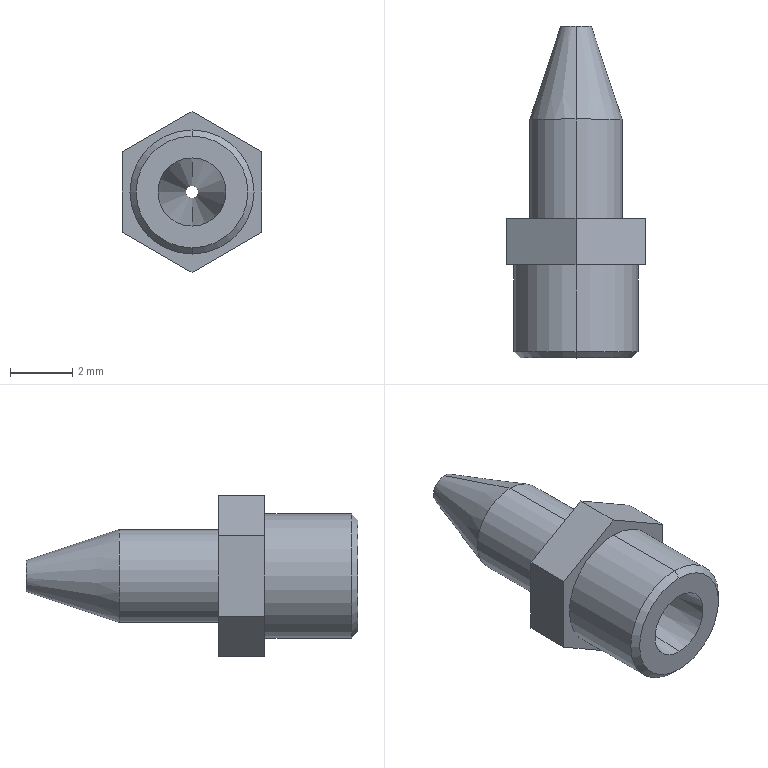Part | SolidWorks | features ICE 4, Chamfer 2, Extrusion 1, RevCut 1 | 1 solid | 20 faces | box 4.5 x 10.7 x 5.196 mm | volume 80.12 mm3 | plane 10 | cone 6 | cylinder 4 | commonest cylinder face diameters 3 x2 4 x2
STEP:
#1=CARTESIAN_POINT('',(0.,-4.5,-1.8));
#2=VERTEX_POINT('',#1);
#3=CARTESIAN_POINT('',(0.,-4.5,1.8));
#4=VERTEX_POINT('',#3);
#5=CARTESIAN_POINT('',(0.,-4.5,0.));
#6=DIRECTION('',(0.,-1.,0.));
#7=DIRECTION('',(0.,0.,-1.));
#8=AXIS2_PLACEMENT_3D('',#5,#6,#7);
#9=CIRCLE('',#8,1.8);
#10=EDGE_CURVE('',#2,#4,#9,.T.);
#11=ORIENTED_EDGE('',*,*,#10,.F.);
#12=CARTESIAN_POINT('',(0.,-4.3,-2.));
#13=VERTEX_POINT('',#12);
#14=CARTESIAN_POINT('',(0.,-4.5,-1.8));
#15=DIRECTION('',(0.,0.7071,-0.7071));
#16=VECTOR('',#15,1000.);
#17=LINE('',#14,#16);
#18=EDGE_CURVE('',#2,#13,#17,.T.);
#19=ORIENTED_EDGE('',*,*,#18,.T.);
#20=CARTESIAN_POINT('',(0.,-4.3,2.));
#21=VERTEX_POINT('',#20);
#22=CARTESIAN_POINT('',(0.,-4.3,0.));
#23=DIRECTION('',(0.,1.,0.));
#24=DIRECTION('',(0.,0.,-1.));
#25=AXIS2_PLACEMENT_3D('',#22,#23,#24);
#26=CIRCLE('',#25,2.);
#27=EDGE_CURVE('',#21,#13,#26,.T.);
#28=ORIENTED_EDGE('',*,*,#27,.F.);
#29=CARTESIAN_POINT('',(0.,-4.5,1.8));
#30=DIRECTION('',(0.,0.7071,0.7071));
#31=VECTOR('',#30,1000.);
#32=LINE('',#29,#31);
#33=EDGE_CURVE('',#4,#21,#32,.T.);
#34=ORIENTED_EDGE('',*,*,#33,.F.);
#35=EDGE_LOOP('',(#11,#19,#28,#34));
#36=FACE_OUTER_BOUND('',#35,.T.);
#37=CARTESIAN_POINT('',(0.,-4.5,0.));
#38=DIRECTION('',(0.,1.,0.));
#39=DIRECTION('',(0.,0.,1.));
#40=AXIS2_PLACEMENT_3D('',#37,#38,#39);
#41=CONICAL_SURFACE('',#40,1.8,0.7854);
#42=ADVANCED_FACE('',(#36),#41,.T.);
#43=CARTESIAN_POINT('',(0.,6.2,0.2));
#44=VERTEX_POINT('',#43);
#45=CARTESIAN_POINT('',(0.,6.2,-0.2));
#46=VERTEX_POINT('',#45);
#47=CARTESIAN_POINT('',(0.,6.2,0.));
#48=DIRECTION('',(0.,-1.,0.));
#49=DIRECTION('',(0.,0.,-1.));
#50=AXIS2_PLACEMENT_3D('',#47,#48,#49);
#51=CIRCLE('',#50,0.2);
#52=EDGE_CURVE('',#44,#46,#51,.T.);
#53=ORIENTED_EDGE('',*,*,#52,.F.);
#54=CARTESIAN_POINT('',(0.,-4.5,1.1));
#55=VERTEX_POINT('',#54);
#56=CARTESIAN_POINT('',(0.,-4.5,1.1));
#57=DIRECTION('',(0.,-0.9965,0.08382));
#58=VECTOR('',#57,1000.);
#59=LINE('',#56,#58);
#60=EDGE_CURVE('',#44,#55,#59,.T.);
#61=ORIENTED_EDGE('',*,*,#60,.T.);
#62=CARTESIAN_POINT('',(0.,-4.5,-1.1));
#63=VERTEX_POINT('',#62);
#64=CARTESIAN_POINT('',(0.,-4.5,0.));
#65=DIRECTION('',(0.,-1.,0.));
#66=DIRECTION('',(0.,0.,-1.));
#67=AXIS2_PLACEMENT_3D('',#64,#65,#66);
#68=CIRCLE('',#67,1.1);
#69=EDGE_CURVE('',#55,#63,#68,.T.);
#70=ORIENTED_EDGE('',*,*,#69,.T.);
#71=CARTESIAN_POINT('',(0.,-4.5,-1.1));
#72=DIRECTION('',(0.,-0.9965,-0.08382));
#73=VECTOR('',#72,1000.);
#74=LINE('',#71,#73);
#75=EDGE_CURVE('',#46,#63,#74,.T.);
#76=ORIENTED_EDGE('',*,*,#75,.F.);
#77=EDGE_LOOP('',(#53,#61,#70,#76));
#78=FACE_OUTER_BOUND('',#77,.T.);
#79=CARTESIAN_POINT('',(0.,-4.5,0.));
#80=DIRECTION('',(0.,-1.,0.));
#81=DIRECTION('',(0.,0.,-1.));
#82=AXIS2_PLACEMENT_3D('',#79,#80,#81);
#83=CONICAL_SURFACE('',#82,1.1,0.08391);
#84=ADVANCED_FACE('',(#78),#83,.F.);
#85=ORIENTED_EDGE('',*,*,#27,.T.);
#86=CARTESIAN_POINT('',(0.,-1.5,-2.));
#87=VERTEX_POINT('',#86);
#88=CARTESIAN_POINT('',(0.,-4.5,-2.));
#89=DIRECTION('',(0.,1.,0.));
#90=VECTOR('',#89,1000.);
#91=LINE('',#88,#90);
#92=EDGE_CURVE('',#13,#87,#91,.T.);
#93=ORIENTED_EDGE('',*,*,#92,.T.);
#94=CARTESIAN_POINT('',(0.,-1.5,2.));
#95=VERTEX_POINT('',#94);
#96=CARTESIAN_POINT('',(0.,-1.5,0.));
#97=DIRECTION('',(0.,-1.,0.));
#98=DIRECTION('',(0.,0.,-1.));
#99=AXIS2_PLACEMENT_3D('',#96,#97,#98);
#100=CIRCLE('',#99,2.);
#101=EDGE_CURVE('',#87,#95,#100,.T.);
#102=ORIENTED_EDGE('',*,*,#101,.T.);
#103=CARTESIAN_POINT('',(0.,-4.5,2.));
#104=DIRECTION('',(0.,1.,0.));
#105=VECTOR('',#104,1000.);
#106=LINE('',#103,#105);
#107=EDGE_CURVE('',#21,#95,#106,.T.);
#108=ORIENTED_EDGE('',*,*,#107,.F.);
#109=EDGE_LOOP('',(#85,#93,#102,#108));
#110=FACE_OUTER_BOUND('',#109,.T.);
#111=CARTESIAN_POINT('',(0.,-4.5,0.));
#112=DIRECTION('',(0.,1.,0.));
#113=DIRECTION('',(0.,0.,1.));
#114=AXIS2_PLACEMENT_3D('',#111,#112,#113);
#115=CYLINDRICAL_SURFACE('',#114,2.);
#116=ADVANCED_FACE('',(#110),#115,.T.);
#117=CARTESIAN_POINT('',(0.,6.2,0.5));
#118=VERTEX_POINT('',#117);
#119=CARTESIAN_POINT('',(0.,6.2,-0.5));
#120=VERTEX_POINT('',#119);
#121=CARTESIAN_POINT('',(0.,6.2,0.));
#122=DIRECTION('',(0.,1.,0.));
#123=DIRECTION('',(0.,0.,1.));
#124=AXIS2_PLACEMENT_3D('',#121,#122,#123);
#125=CIRCLE('',#124,0.5);
#126=EDGE_CURVE('',#118,#120,#125,.T.);
#127=ORIENTED_EDGE('',*,*,#126,.F.);
#128=CARTESIAN_POINT('',(0.,3.2,1.5));
#129=VERTEX_POINT('',#128);
#130=CARTESIAN_POINT('',(0.,6.2,0.5));
#131=DIRECTION('',(0.,-0.9487,0.3162));
#132=VECTOR('',#131,1000.);
#133=LINE('',#130,#132);
#134=EDGE_CURVE('',#118,#129,#133,.T.);
#135=ORIENTED_EDGE('',*,*,#134,.T.);
#136=CARTESIAN_POINT('',(0.,3.2,-1.5));
#137=VERTEX_POINT('',#136);
#138=CARTESIAN_POINT('',(0.,3.2,0.));
#139=DIRECTION('',(0.,-1.,0.));
#140=DIRECTION('',(0.,0.,1.));
#141=AXIS2_PLACEMENT_3D('',#138,#139,#140);
#142=CIRCLE('',#141,1.5);
#143=EDGE_CURVE('',#137,#129,#142,.T.);
#144=ORIENTED_EDGE('',*,*,#143,.F.);
#145=CARTESIAN_POINT('',(0.,6.2,-0.5));
#146=DIRECTION('',(0.,-0.9487,-0.3162));
#147=VECTOR('',#146,1000.);
#148=LINE('',#145,#147);
#149=EDGE_CURVE('',#120,#137,#148,.T.);
#150=ORIENTED_EDGE('',*,*,#149,.F.);
#151=EDGE_LOOP('',(#127,#135,#144,#150));
#152=FACE_OUTER_BOUND('',#151,.T.);
#153=CARTESIAN_POINT('',(0.,6.2,0.));
#154=DIRECTION('',(0.,-1.,0.));
#155=DIRECTION('',(0.,0.,-1.));
#156=AXIS2_PLACEMENT_3D('',#153,#154,#155);
#157=CONICAL_SURFACE('',#156,0.5,0.3218);
#158=ADVANCED_FACE('',(#152),#157,.T.);
#159=ORIENTED_EDGE('',*,*,#143,.T.);
#160=CARTESIAN_POINT('',(0.,0.,1.5));
#161=VERTEX_POINT('',#160);
#162=CARTESIAN_POINT('',(0.,6.2,1.5));
#163=DIRECTION('',(0.,-1.,0.));
#164=VECTOR('',#163,1000.);
#165=LINE('',#162,#164);
#166=EDGE_CURVE('',#129,#161,#165,.T.);
#167=ORIENTED_EDGE('',*,*,#166,.T.);
#168=CARTESIAN_POINT('',(0.,0.,-1.5));
#169=VERTEX_POINT('',#168);
#170=CARTESIAN_POINT('',(0.,0.,0.));
#171=DIRECTION('',(0.,-1.,0.));
#172=DIRECTION('',(0.,0.,-1.));
#173=AXIS2_PLACEMENT_3D('',#170,#171,#172);
#174=CIRCLE('',#173,1.5);
#175=EDGE_CURVE('',#169,#161,#174,.T.);
#176=ORIENTED_EDGE('',*,*,#175,.F.);
#177=CARTESIAN_POINT('',(0.,6.2,-1.5));
#178=DIRECTION('',(0.,-1.,0.));
#179=VECTOR('',#178,1000.);
#180=LINE('',#177,#179);
#181=EDGE_CURVE('',#137,#169,#180,.T.);
#182=ORIENTED_EDGE('',*,*,#181,.F.);
#183=EDGE_LOOP('',(#159,#167,#176,#182));
#184=FACE_OUTER_BOUND('',#183,.T.);
#185=CARTESIAN_POINT('',(0.,6.2,0.));
#186=DIRECTION('',(0.,-1.,0.));
#187=DIRECTION('',(0.,0.,-1.));
#188=AXIS2_PLACEMENT_3D('',#185,#186,#187);
#189=CYLINDRICAL_SURFACE('',#188,1.5);
#190=ADVANCED_FACE('',(#184),#189,.T.);
#191=CARTESIAN_POINT('',(2.25,-1.5,1.299));
#192=VERTEX_POINT('',#191);
#193=CARTESIAN_POINT('',(0.,-1.5,2.598));
#194=VERTEX_POINT('',#193);
#195=CARTESIAN_POINT('',(2.25,-1.5,1.299));
#196=DIRECTION('',(-0.866,0.,0.5));
#197=VECTOR('',#196,1000.);
#198=LINE('',#195,#197);
#199=EDGE_CURVE('',#192,#194,#198,.T.);
#200=ORIENTED_EDGE('',*,*,#199,.T.);
#201=CARTESIAN_POINT('',(-2.25,-1.5,1.299));
#202=VERTEX_POINT('',#201);
#203=CARTESIAN_POINT('',(0.,-1.5,2.598));
#204=DIRECTION('',(-0.866,0.,-0.5));
#205=VECTOR('',#204,1000.);
#206=LINE('',#203,#205);
#207=EDGE_CURVE('',#194,#202,#206,.T.);
#208=ORIENTED_EDGE('',*,*,#207,.T.);
#209=CARTESIAN_POINT('',(-2.25,-1.5,-1.299));
#210=VERTEX_POINT('',#209);
#211=CARTESIAN_POINT('',(-2.25,-1.5,1.299));
#212=DIRECTION('',(0.,0.,-1.));
#213=VECTOR('',#212,1000.);
#214=LINE('',#211,#213);
#215=EDGE_CURVE('',#202,#210,#214,.T.);
#216=ORIENTED_EDGE('',*,*,#215,.T.);
#217=CARTESIAN_POINT('',(0.,-1.5,-2.598));
#218=VERTEX_POINT('',#217);
#219=CARTESIAN_POINT('',(-2.25,-1.5,-1.299));
#220=DIRECTION('',(0.866,0.,-0.5));
#221=VECTOR('',#220,1000.);
#222=LINE('',#219,#221);
#223=EDGE_CURVE('',#210,#218,#222,.T.);
#224=ORIENTED_EDGE('',*,*,#223,.T.);
#225=CARTESIAN_POINT('',(2.25,-1.5,-1.299));
#226=VERTEX_POINT('',#225);
#227=CARTESIAN_POINT('',(0.,-1.5,-2.598));
#228=DIRECTION('',(0.866,0.,0.5));
#229=VECTOR('',#228,1000.);
#230=LINE('',#227,#229);
#231=EDGE_CURVE('',#218,#226,#230,.T.);
#232=ORIENTED_EDGE('',*,*,#231,.T.);
#233=CARTESIAN_POINT('',(2.25,-1.5,-1.299));
#234=DIRECTION('',(0.,0.,1.));
#235=VECTOR('',#234,1000.);
#236=LINE('',#233,#235);
#237=EDGE_CURVE('',#226,#192,#236,.T.);
#238=ORIENTED_EDGE('',*,*,#237,.T.);
#239=EDGE_LOOP('',(#200,#208,#216,#224,#232,#238));
#240=FACE_OUTER_BOUND('',#239,.T.);
#241=CARTESIAN_POINT('',(0.,-1.5,0.));
#242=DIRECTION('',(0.,-1.,0.));
#243=DIRECTION('',(0.,0.,-1.));
#244=AXIS2_PLACEMENT_3D('',#241,#242,#243);
#245=CIRCLE('',#244,2.);
#246=EDGE_CURVE('',#95,#87,#245,.T.);
#247=ORIENTED_EDGE('',*,*,#246,.F.);
#248=ORIENTED_EDGE('',*,*,#101,.F.);
#249=EDGE_LOOP('',(#247,#248));
#250=FACE_BOUND('',#249,.T.);
#251=CARTESIAN_POINT('',(0.,-1.5,0.));
#252=DIRECTION('',(0.,-1.,0.));
#253=DIRECTION('',(0.,0.,-1.));
#254=AXIS2_PLACEMENT_3D('',#251,#252,#253);
#255=PLANE('',#254);
#256=ADVANCED_FACE('',(#240,#250),#255,.T.);
#257=ORIENTED_EDGE('',*,*,#166,.F.);
#258=CARTESIAN_POINT('',(0.,3.2,0.));
#259=DIRECTION('',(0.,-1.,0.));
#260=DIRECTION('',(0.,0.,1.));
#261=AXIS2_PLACEMENT_3D('',#258,#259,#260);
#262=CIRCLE('',#261,1.5);
#263=EDGE_CURVE('',#129,#137,#262,.T.);
#264=ORIENTED_EDGE('',*,*,#263,.T.);
#265=ORIENTED_EDGE('',*,*,#181,.T.);
#266=CARTESIAN_POINT('',(0.,0.,0.));
#267=DIRECTION('',(0.,-1.,0.));
#268=DIRECTION('',(0.,0.,-1.));
#269=AXIS2_PLACEMENT_3D('',#266,#267,#268);
#270=CIRCLE('',#269,1.5);
#271=EDGE_CURVE('',#161,#169,#270,.T.);
#272=ORIENTED_EDGE('',*,*,#271,.F.);
#273=EDGE_LOOP('',(#257,#264,#265,#272));
#274=FACE_OUTER_BOUND('',#273,.T.);
#275=CARTESIAN_POINT('',(0.,6.2,0.));
#276=DIRECTION('',(0.,-1.,0.));
#277=DIRECTION('',(0.,0.,-1.));
#278=AXIS2_PLACEMENT_3D('',#275,#276,#277);
#279=CYLINDRICAL_SURFACE('',#278,1.5);
#280=ADVANCED_FACE('',(#274),#279,.T.);
#281=CARTESIAN_POINT('',(0.,6.2,0.));
#282=DIRECTION('',(0.,1.,0.));
#283=DIRECTION('',(0.,0.,1.));
#284=AXIS2_PLACEMENT_3D('',#281,#282,#283);
#285=CIRCLE('',#284,0.5);
#286=EDGE_CURVE('',#120,#118,#285,.T.);
#287=ORIENTED_EDGE('',*,*,#286,.T.);
#288=ORIENTED_EDGE('',*,*,#126,.T.);
#289=EDGE_LOOP('',(#287,#288));
#290=FACE_OUTER_BOUND('',#289,.T.);
#291=CARTESIAN_POINT('',(0.,6.2,0.));
#292=DIRECTION('',(0.,-1.,0.));
#293=DIRECTION('',(0.,0.,-1.));
#294=AXIS2_PLACEMENT_3D('',#291,#292,#293);
#295=CIRCLE('',#294,0.2);
#296=EDGE_CURVE('',#46,#44,#295,.T.);
#297=ORIENTED_EDGE('',*,*,#296,.T.);
#298=ORIENTED_EDGE('',*,*,#52,.T.);
#299=EDGE_LOOP('',(#297,#298));
#300=FACE_BOUND('',#299,.T.);
#301=CARTESIAN_POINT('',(0.,6.2,0.));
#302=DIRECTION('',(0.,1.,0.));
#303=DIRECTION('',(0.,0.,1.));
#304=AXIS2_PLACEMENT_3D('',#301,#302,#303);
#305=PLANE('',#304);
#306=ADVANCED_FACE('',(#290,#300),#305,.T.);
#307=ORIENTED_EDGE('',*,*,#134,.F.);
#308=ORIENTED_EDGE('',*,*,#286,.F.);
#309=ORIENTED_EDGE('',*,*,#149,.T.);
#310=ORIENTED_EDGE('',*,*,#263,.F.);
#311=EDGE_LOOP('',(#307,#308,#309,#310));
#312=FACE_OUTER_BOUND('',#311,.T.);
#313=CARTESIAN_POINT('',(0.,6.2,0.));
#314=DIRECTION('',(0.,-1.,0.));
#315=DIRECTION('',(0.,0.,-1.));
#316=AXIS2_PLACEMENT_3D('',#313,#314,#315);
#317=CONICAL_SURFACE('',#316,0.5,0.3218);
#318=ADVANCED_FACE('',(#312),#317,.T.);
#319=CARTESIAN_POINT('',(2.25,0.,1.299));
#320=VERTEX_POINT('',#319);
#321=CARTESIAN_POINT('',(0.,0.,2.598));
#322=VERTEX_POINT('',#321);
#323=CARTESIAN_POINT('',(2.25,0.,1.299));
#324=DIRECTION('',(-0.866,0.,0.5));
#325=VECTOR('',#324,1000.);
#326=LINE('',#323,#325);
#327=EDGE_CURVE('',#320,#322,#326,.T.);
#328=ORIENTED_EDGE('',*,*,#327,.F.);
#329=CARTESIAN_POINT('',(2.25,0.,-1.299));
#330=VERTEX_POINT('',#329);
#331=CARTESIAN_POINT('',(2.25,0.,-1.299));
#332=DIRECTION('',(0.,0.,1.));
#333=VECTOR('',#332,1000.);
#334=LINE('',#331,#333);
#335=EDGE_CURVE('',#330,#320,#334,.T.);
#336=ORIENTED_EDGE('',*,*,#335,.F.);
#337=CARTESIAN_POINT('',(0.,0.,-2.598));
#338=VERTEX_POINT('',#337);
#339=CARTESIAN_POINT('',(0.,0.,-2.598));
#340=DIRECTION('',(0.866,0.,0.5));
#341=VECTOR('',#340,1000.);
#342=LINE('',#339,#341);
#343=EDGE_CURVE('',#338,#330,#342,.T.);
#344=ORIENTED_EDGE('',*,*,#343,.F.);
#345=CARTESIAN_POINT('',(-2.25,0.,-1.299));
#346=VERTEX_POINT('',#345);
#347=CARTESIAN_POINT('',(-2.25,0.,-1.299));
#348=DIRECTION('',(0.866,0.,-0.5));
#349=VECTOR('',#348,1000.);
#350=LINE('',#347,#349);
#351=EDGE_CURVE('',#346,#338,#350,.T.);
#352=ORIENTED_EDGE('',*,*,#351,.F.);
#353=CARTESIAN_POINT('',(-2.25,0.,1.299));
#354=VERTEX_POINT('',#353);
#355=CARTESIAN_POINT('',(-2.25,0.,1.299));
#356=DIRECTION('',(0.,0.,-1.));
#357=VECTOR('',#356,1000.);
#358=LINE('',#355,#357);
#359=EDGE_CURVE('',#354,#346,#358,.T.);
#360=ORIENTED_EDGE('',*,*,#359,.F.);
#361=CARTESIAN_POINT('',(0.,0.,2.598));
#362=DIRECTION('',(-0.866,0.,-0.5));
#363=VECTOR('',#362,1000.);
#364=LINE('',#361,#363);
#365=EDGE_CURVE('',#322,#354,#364,.T.);
#366=ORIENTED_EDGE('',*,*,#365,.F.);
#367=EDGE_LOOP('',(#328,#336,#344,#352,#360,#366));
#368=FACE_OUTER_BOUND('',#367,.T.);
#369=ORIENTED_EDGE('',*,*,#175,.T.);
#370=ORIENTED_EDGE('',*,*,#271,.T.);
#371=EDGE_LOOP('',(#369,#370));
#372=FACE_BOUND('',#371,.T.);
#373=CARTESIAN_POINT('',(0.,0.,0.));
#374=DIRECTION('',(0.,-1.,0.));
#375=DIRECTION('',(0.,0.,-1.));
#376=AXIS2_PLACEMENT_3D('',#373,#374,#375);
#377=PLANE('',#376);
#378=ADVANCED_FACE('',(#368,#372),#377,.F.);
#379=ORIENTED_EDGE('',*,*,#327,.T.);
#380=CARTESIAN_POINT('',(0.,-1.5,2.598));
#381=DIRECTION('',(0.,1.,0.));
#382=VECTOR('',#381,1000.);
#383=LINE('',#380,#382);
#384=EDGE_CURVE('',#194,#322,#383,.T.);
#385=ORIENTED_EDGE('',*,*,#384,.F.);
#386=ORIENTED_EDGE('',*,*,#199,.F.);
#387=CARTESIAN_POINT('',(2.25,-1.5,1.299));
#388=DIRECTION('',(0.,1.,0.));
#389=VECTOR('',#388,1000.);
#390=LINE('',#387,#389);
#391=EDGE_CURVE('',#192,#320,#390,.T.);
#392=ORIENTED_EDGE('',*,*,#391,.T.);
#393=EDGE_LOOP('',(#379,#385,#386,#392));
#394=FACE_OUTER_BOUND('',#393,.T.);
#395=CARTESIAN_POINT('',(2.25,-1.5,1.299));
#396=DIRECTION('',(-0.5,0.,-0.866));
#397=DIRECTION('',(-0.866,0.,0.5));
#398=AXIS2_PLACEMENT_3D('',#395,#396,#397);
#399=PLANE('',#398);
#400=ADVANCED_FACE('',(#394),#399,.F.);
#401=ORIENTED_EDGE('',*,*,#365,.T.);
#402=CARTESIAN_POINT('',(-2.25,-1.5,1.299));
#403=DIRECTION('',(0.,1.,0.));
#404=VECTOR('',#403,1000.);
#405=LINE('',#402,#404);
#406=EDGE_CURVE('',#202,#354,#405,.T.);
#407=ORIENTED_EDGE('',*,*,#406,.F.);
#408=ORIENTED_EDGE('',*,*,#207,.F.);
#409=ORIENTED_EDGE('',*,*,#384,.T.);
#410=EDGE_LOOP('',(#401,#407,#408,#409));
#411=FACE_OUTER_BOUND('',#410,.T.);
#412=CARTESIAN_POINT('',(0.,-1.5,2.598));
#413=DIRECTION('',(0.5,0.,-0.866));
#414=DIRECTION('',(-0.866,0.,-0.5));
#415=AXIS2_PLACEMENT_3D('',#412,#413,#414);
#416=PLANE('',#415);
#417=ADVANCED_FACE('',(#411),#416,.F.);
#418=ORIENTED_EDGE('',*,*,#359,.T.);
#419=CARTESIAN_POINT('',(-2.25,-1.5,-1.299));
#420=DIRECTION('',(0.,1.,0.));
#421=VECTOR('',#420,1000.);
#422=LINE('',#419,#421);
#423=EDGE_CURVE('',#210,#346,#422,.T.);
#424=ORIENTED_EDGE('',*,*,#423,.F.);
#425=ORIENTED_EDGE('',*,*,#215,.F.);
#426=ORIENTED_EDGE('',*,*,#406,.T.);
#427=EDGE_LOOP('',(#418,#424,#425,#426));
#428=FACE_OUTER_BOUND('',#427,.T.);
#429=CARTESIAN_POINT('',(-2.25,-1.5,1.299));
#430=DIRECTION('',(1.,0.,0.));
#431=DIRECTION('',(0.,0.,-1.));
#432=AXIS2_PLACEMENT_3D('',#429,#430,#431);
#433=PLANE('',#432);
#434=ADVANCED_FACE('',(#428),#433,.F.);
#435=ORIENTED_EDGE('',*,*,#351,.T.);
#436=CARTESIAN_POINT('',(0.,-1.5,-2.598));
#437=DIRECTION('',(0.,1.,0.));
#438=VECTOR('',#437,1000.);
#439=LINE('',#436,#438);
#440=EDGE_CURVE('',#218,#338,#439,.T.);
#441=ORIENTED_EDGE('',*,*,#440,.F.);
#442=ORIENTED_EDGE('',*,*,#223,.F.);
#443=ORIENTED_EDGE('',*,*,#423,.T.);
#444=EDGE_LOOP('',(#435,#441,#442,#443));
#445=FACE_OUTER_BOUND('',#444,.T.);
#446=CARTESIAN_POINT('',(-2.25,-1.5,-1.299));
#447=DIRECTION('',(0.5,0.,0.866));
#448=DIRECTION('',(0.866,0.,-0.5));
#449=AXIS2_PLACEMENT_3D('',#446,#447,#448);
#450=PLANE('',#449);
#451=ADVANCED_FACE('',(#445),#450,.F.);
#452=ORIENTED_EDGE('',*,*,#343,.T.);
#453=CARTESIAN_POINT('',(2.25,-1.5,-1.299));
#454=DIRECTION('',(0.,1.,0.));
#455=VECTOR('',#454,1000.);
#456=LINE('',#453,#455);
#457=EDGE_CURVE('',#226,#330,#456,.T.);
#458=ORIENTED_EDGE('',*,*,#457,.F.);
#459=ORIENTED_EDGE('',*,*,#231,.F.);
#460=ORIENTED_EDGE('',*,*,#440,.T.);
#461=EDGE_LOOP('',(#452,#458,#459,#460));
#462=FACE_OUTER_BOUND('',#461,.T.);
#463=CARTESIAN_POINT('',(0.,-1.5,-2.598));
#464=DIRECTION('',(-0.5,0.,0.866));
#465=DIRECTION('',(0.866,0.,0.5));
#466=AXIS2_PLACEMENT_3D('',#463,#464,#465);
#467=PLANE('',#466);
#468=ADVANCED_FACE('',(#462),#467,.F.);
#469=ORIENTED_EDGE('',*,*,#335,.T.);
#470=ORIENTED_EDGE('',*,*,#391,.F.);
#471=ORIENTED_EDGE('',*,*,#237,.F.);
#472=ORIENTED_EDGE('',*,*,#457,.T.);
#473=EDGE_LOOP('',(#469,#470,#471,#472));
#474=FACE_OUTER_BOUND('',#473,.T.);
#475=CARTESIAN_POINT('',(2.25,-1.5,-1.299));
#476=DIRECTION('',(-1.,0.,0.));
#477=DIRECTION('',(0.,0.,1.));
#478=AXIS2_PLACEMENT_3D('',#475,#476,#477);
#479=PLANE('',#478);
#480=ADVANCED_FACE('',(#474),#479,.F.);
#481=CARTESIAN_POINT('',(0.,-4.5,0.));
#482=DIRECTION('',(0.,-1.,0.));
#483=DIRECTION('',(0.,0.,-1.));
#484=AXIS2_PLACEMENT_3D('',#481,#482,#483);
#485=CIRCLE('',#484,1.8);
#486=EDGE_CURVE('',#4,#2,#485,.T.);
#487=ORIENTED_EDGE('',*,*,#486,.T.);
#488=ORIENTED_EDGE('',*,*,#10,.T.);
#489=EDGE_LOOP('',(#487,#488));
#490=FACE_OUTER_BOUND('',#489,.T.);
#491=CARTESIAN_POINT('',(0.,-4.5,0.));
#492=DIRECTION('',(0.,-1.,0.));
#493=DIRECTION('',(0.,0.,-1.));
#494=AXIS2_PLACEMENT_3D('',#491,#492,#493);
#495=CIRCLE('',#494,1.1);
#496=EDGE_CURVE('',#63,#55,#495,.T.);
#497=ORIENTED_EDGE('',*,*,#496,.F.);
#498=ORIENTED_EDGE('',*,*,#69,.F.);
#499=EDGE_LOOP('',(#497,#498));
#500=FACE_BOUND('',#499,.T.);
#501=CARTESIAN_POINT('',(0.,-4.5,0.));
#502=DIRECTION('',(0.,-1.,0.));
#503=DIRECTION('',(0.,0.,-1.));
#504=AXIS2_PLACEMENT_3D('',#501,#502,#503);
#505=PLANE('',#504);
#506=ADVANCED_FACE('',(#490,#500),#505,.T.);
#507=ORIENTED_EDGE('',*,*,#92,.F.);
#508=CARTESIAN_POINT('',(0.,-4.3,0.));
#509=DIRECTION('',(0.,1.,0.));
#510=DIRECTION('',(0.,0.,-1.));
#511=AXIS2_PLACEMENT_3D('',#508,#509,#510);
#512=CIRCLE('',#511,2.);
#513=EDGE_CURVE('',#13,#21,#512,.T.);
#514=ORIENTED_EDGE('',*,*,#513,.T.);
#515=ORIENTED_EDGE('',*,*,#107,.T.);
#516=ORIENTED_EDGE('',*,*,#246,.T.);
#517=EDGE_LOOP('',(#507,#514,#515,#516));
#518=FACE_OUTER_BOUND('',#517,.T.);
#519=CARTESIAN_POINT('',(0.,-4.5,0.));
#520=DIRECTION('',(0.,1.,0.));
#521=DIRECTION('',(0.,0.,1.));
#522=AXIS2_PLACEMENT_3D('',#519,#520,#521);
#523=CYLINDRICAL_SURFACE('',#522,2.);
#524=ADVANCED_FACE('',(#518),#523,.T.);
#525=ORIENTED_EDGE('',*,*,#60,.F.);
#526=ORIENTED_EDGE('',*,*,#296,.F.);
#527=ORIENTED_EDGE('',*,*,#75,.T.);
#528=ORIENTED_EDGE('',*,*,#496,.T.);
#529=EDGE_LOOP('',(#525,#526,#527,#528));
#530=FACE_OUTER_BOUND('',#529,.T.);
#531=CARTESIAN_POINT('',(0.,-4.5,0.));
#532=DIRECTION('',(0.,-1.,0.));
#533=DIRECTION('',(0.,0.,-1.));
#534=AXIS2_PLACEMENT_3D('',#531,#532,#533);
#535=CONICAL_SURFACE('',#534,1.1,0.08391);
#536=ADVANCED_FACE('',(#530),#535,.F.);
#537=ORIENTED_EDGE('',*,*,#18,.F.);
#538=ORIENTED_EDGE('',*,*,#486,.F.);
#539=ORIENTED_EDGE('',*,*,#33,.T.);
#540=ORIENTED_EDGE('',*,*,#513,.F.);
#541=EDGE_LOOP('',(#537,#538,#539,#540));
#542=FACE_OUTER_BOUND('',#541,.T.);
#543=CARTESIAN_POINT('',(0.,-4.5,0.));
#544=DIRECTION('',(0.,1.,0.));
#545=DIRECTION('',(0.,0.,1.));
#546=AXIS2_PLACEMENT_3D('',#543,#544,#545);
#547=CONICAL_SURFACE('',#546,1.8,0.7854);
#548=ADVANCED_FACE('',(#542),#547,.T.);
#549=CLOSED_SHELL('',(#42,#84,#116,#158,#190,#256,#280,#306,#318,#378,#400,#417,#434,#451,#468,#480,#506,#524,#536,#548));
#550=MANIFOLD_SOLID_BREP('',#549);
#551=CARTESIAN_POINT('',(0.,0.,0.));
#552=DIRECTION('',(0.,0.,1.));
#553=DIRECTION('',(1.,0.,0.));
#554=AXIS2_PLACEMENT_3D('',#551,#552,#553);
#555=(LENGTH_UNIT()NAMED_UNIT(*)SI_UNIT(.MILLI.,.METRE.));
#556=UNCERTAINTY_MEASURE_WITH_UNIT(LENGTH_MEASURE(0.00001),#555,'','');
#557=(NAMED_UNIT(*)PLANE_ANGLE_UNIT()SI_UNIT($,.RADIAN.));
#558=(NAMED_UNIT(*)SI_UNIT($,.STERADIAN.)SOLID_ANGLE_UNIT());
#559=(GEOMETRIC_REPRESENTATION_CONTEXT(3)GLOBAL_UNCERTAINTY_ASSIGNED_CONTEXT((#556))GLOBAL_UNIT_ASSIGNED_CONTEXT((#555,#557,#558))REPRESENTATION_CONTEXT('',''));
#560=ADVANCED_BREP_SHAPE_REPRESENTATION('',(#550,#554),#559);